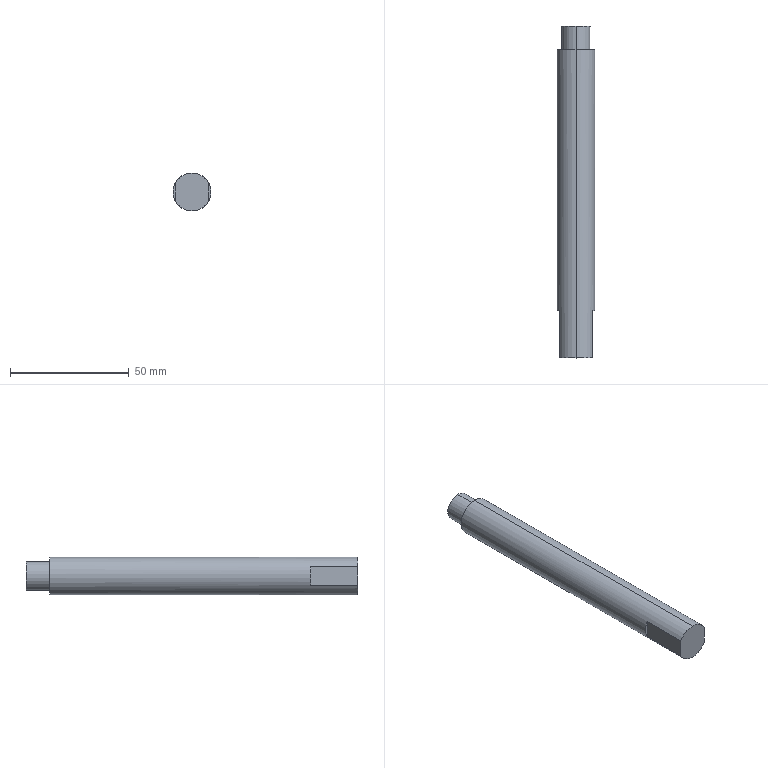Part | SolidWorks | features ICE 2, Extrusion 1, HoleWzd 1 | 1 solid | 11 faces | box 16 x 140 x 16 mm | volume 27060 mm3 | plane 7 | cylinder 4 | commonest cylinder face diameters 12 x2 16 x2
STEP:
#1=CARTESIAN_POINT('',(0.,140.,6.));
#2=VERTEX_POINT('',#1);
#3=CARTESIAN_POINT('',(0.,140.,-6.));
#4=VERTEX_POINT('',#3);
#5=CARTESIAN_POINT('',(0.,140.,0.));
#6=DIRECTION('',(0.,1.,0.));
#7=DIRECTION('',(0.,0.,1.));
#8=AXIS2_PLACEMENT_3D('',#5,#6,#7);
#9=CIRCLE('',#8,6.);
#10=EDGE_CURVE('',#2,#4,#9,.T.);
#11=ORIENTED_EDGE('',*,*,#10,.F.);
#12=CARTESIAN_POINT('',(0.,130.,6.));
#13=VERTEX_POINT('',#12);
#14=CARTESIAN_POINT('',(0.,140.,6.));
#15=DIRECTION('',(0.,-1.,0.));
#16=VECTOR('',#15,1000.);
#17=LINE('',#14,#16);
#18=EDGE_CURVE('',#2,#13,#17,.T.);
#19=ORIENTED_EDGE('',*,*,#18,.T.);
#20=CARTESIAN_POINT('',(0.,130.,-6.));
#21=VERTEX_POINT('',#20);
#22=CARTESIAN_POINT('',(0.,130.,0.));
#23=DIRECTION('',(0.,1.,0.));
#24=DIRECTION('',(0.,0.,1.));
#25=AXIS2_PLACEMENT_3D('',#22,#23,#24);
#26=CIRCLE('',#25,6.);
#27=EDGE_CURVE('',#13,#21,#26,.T.);
#28=ORIENTED_EDGE('',*,*,#27,.T.);
#29=CARTESIAN_POINT('',(0.,140.,-6.));
#30=DIRECTION('',(0.,-1.,0.));
#31=VECTOR('',#30,1000.);
#32=LINE('',#29,#31);
#33=EDGE_CURVE('',#4,#21,#32,.T.);
#34=ORIENTED_EDGE('',*,*,#33,.F.);
#35=EDGE_LOOP('',(#11,#19,#28,#34));
#36=FACE_OUTER_BOUND('',#35,.T.);
#37=CARTESIAN_POINT('',(0.,140.,0.));
#38=DIRECTION('',(0.,-1.,0.));
#39=DIRECTION('',(0.,0.,-1.));
#40=AXIS2_PLACEMENT_3D('',#37,#38,#39);
#41=CYLINDRICAL_SURFACE('',#40,6.);
#42=ADVANCED_FACE('',(#36),#41,.T.);
#43=CARTESIAN_POINT('',(0.,130.,8.));
#44=VERTEX_POINT('',#43);
#45=CARTESIAN_POINT('',(0.,130.,-8.));
#46=VERTEX_POINT('',#45);
#47=CARTESIAN_POINT('',(0.,130.,0.));
#48=DIRECTION('',(0.,1.,0.));
#49=DIRECTION('',(0.,0.,1.));
#50=AXIS2_PLACEMENT_3D('',#47,#48,#49);
#51=CIRCLE('',#50,8.);
#52=EDGE_CURVE('',#44,#46,#51,.T.);
#53=ORIENTED_EDGE('',*,*,#52,.F.);
#54=CARTESIAN_POINT('',(0.,0.,8.));
#55=VERTEX_POINT('',#54);
#56=CARTESIAN_POINT('',(0.,130.,8.));
#57=DIRECTION('',(0.,-1.,0.));
#58=VECTOR('',#57,1000.);
#59=LINE('',#56,#58);
#60=EDGE_CURVE('',#44,#55,#59,.T.);
#61=ORIENTED_EDGE('',*,*,#60,.T.);
#62=CARTESIAN_POINT('',(7.,0.,3.873));
#63=VERTEX_POINT('',#62);
#64=CARTESIAN_POINT('',(0.,0.,0.));
#65=DIRECTION('',(0.,1.,0.));
#66=DIRECTION('',(0.,0.,1.));
#67=AXIS2_PLACEMENT_3D('',#64,#65,#66);
#68=CIRCLE('',#67,8.);
#69=EDGE_CURVE('',#55,#63,#68,.T.);
#70=ORIENTED_EDGE('',*,*,#69,.T.);
#71=CARTESIAN_POINT('',(7.,20.,3.873));
#72=VERTEX_POINT('',#71);
#73=CARTESIAN_POINT('',(7.,130.,3.873));
#74=DIRECTION('',(0.,1.,0.));
#75=VECTOR('',#74,1000.);
#76=LINE('',#73,#75);
#77=EDGE_CURVE('',#63,#72,#76,.T.);
#78=ORIENTED_EDGE('',*,*,#77,.T.);
#79=CARTESIAN_POINT('',(7.,20.,-3.873));
#80=VERTEX_POINT('',#79);
#81=CARTESIAN_POINT('',(0.,20.,0.));
#82=DIRECTION('',(0.,1.,0.));
#83=DIRECTION('',(-1.,0.,0.));
#84=AXIS2_PLACEMENT_3D('',#81,#82,#83);
#85=CIRCLE('',#84,8.);
#86=EDGE_CURVE('',#72,#80,#85,.T.);
#87=ORIENTED_EDGE('',*,*,#86,.T.);
#88=CARTESIAN_POINT('',(7.,0.,-3.873));
#89=VERTEX_POINT('',#88);
#90=CARTESIAN_POINT('',(7.,130.,-3.873));
#91=DIRECTION('',(0.,-1.,0.));
#92=VECTOR('',#91,1000.);
#93=LINE('',#90,#92);
#94=EDGE_CURVE('',#80,#89,#93,.T.);
#95=ORIENTED_EDGE('',*,*,#94,.T.);
#96=CARTESIAN_POINT('',(0.,0.,-8.));
#97=VERTEX_POINT('',#96);
#98=CARTESIAN_POINT('',(0.,0.,0.));
#99=DIRECTION('',(0.,1.,0.));
#100=DIRECTION('',(0.,0.,1.));
#101=AXIS2_PLACEMENT_3D('',#98,#99,#100);
#102=CIRCLE('',#101,8.);
#103=EDGE_CURVE('',#89,#97,#102,.T.);
#104=ORIENTED_EDGE('',*,*,#103,.T.);
#105=CARTESIAN_POINT('',(0.,130.,-8.));
#106=DIRECTION('',(0.,-1.,0.));
#107=VECTOR('',#106,1000.);
#108=LINE('',#105,#107);
#109=EDGE_CURVE('',#46,#97,#108,.T.);
#110=ORIENTED_EDGE('',*,*,#109,.F.);
#111=EDGE_LOOP('',(#53,#61,#70,#78,#87,#95,#104,#110));
#112=FACE_OUTER_BOUND('',#111,.T.);
#113=CARTESIAN_POINT('',(0.,130.,0.));
#114=DIRECTION('',(0.,-1.,0.));
#115=DIRECTION('',(0.,0.,-1.));
#116=AXIS2_PLACEMENT_3D('',#113,#114,#115);
#117=CYLINDRICAL_SURFACE('',#116,8.);
#118=ADVANCED_FACE('',(#112),#117,.T.);
#119=ORIENTED_EDGE('',*,*,#60,.F.);
#120=CARTESIAN_POINT('',(0.,130.,0.));
#121=DIRECTION('',(0.,1.,0.));
#122=DIRECTION('',(0.,0.,1.));
#123=AXIS2_PLACEMENT_3D('',#120,#121,#122);
#124=CIRCLE('',#123,8.);
#125=EDGE_CURVE('',#46,#44,#124,.T.);
#126=ORIENTED_EDGE('',*,*,#125,.F.);
#127=ORIENTED_EDGE('',*,*,#109,.T.);
#128=CARTESIAN_POINT('',(-7.,0.,-3.873));
#129=VERTEX_POINT('',#128);
#130=CARTESIAN_POINT('',(0.,0.,0.));
#131=DIRECTION('',(0.,1.,0.));
#132=DIRECTION('',(0.,0.,1.));
#133=AXIS2_PLACEMENT_3D('',#130,#131,#132);
#134=CIRCLE('',#133,8.);
#135=EDGE_CURVE('',#97,#129,#134,.T.);
#136=ORIENTED_EDGE('',*,*,#135,.T.);
#137=CARTESIAN_POINT('',(-7.,20.,-3.873));
#138=VERTEX_POINT('',#137);
#139=CARTESIAN_POINT('',(-7.,130.,-3.873));
#140=DIRECTION('',(0.,1.,0.));
#141=VECTOR('',#140,1000.);
#142=LINE('',#139,#141);
#143=EDGE_CURVE('',#129,#138,#142,.T.);
#144=ORIENTED_EDGE('',*,*,#143,.T.);
#145=CARTESIAN_POINT('',(-7.,20.,3.873));
#146=VERTEX_POINT('',#145);
#147=CARTESIAN_POINT('',(0.,20.,0.));
#148=DIRECTION('',(0.,1.,0.));
#149=DIRECTION('',(-1.,0.,0.));
#150=AXIS2_PLACEMENT_3D('',#147,#148,#149);
#151=CIRCLE('',#150,8.);
#152=EDGE_CURVE('',#138,#146,#151,.T.);
#153=ORIENTED_EDGE('',*,*,#152,.T.);
#154=CARTESIAN_POINT('',(-7.,0.,3.873));
#155=VERTEX_POINT('',#154);
#156=CARTESIAN_POINT('',(-7.,130.,3.873));
#157=DIRECTION('',(0.,-1.,0.));
#158=VECTOR('',#157,1000.);
#159=LINE('',#156,#158);
#160=EDGE_CURVE('',#146,#155,#159,.T.);
#161=ORIENTED_EDGE('',*,*,#160,.T.);
#162=CARTESIAN_POINT('',(0.,0.,0.));
#163=DIRECTION('',(0.,1.,0.));
#164=DIRECTION('',(0.,0.,1.));
#165=AXIS2_PLACEMENT_3D('',#162,#163,#164);
#166=CIRCLE('',#165,8.);
#167=EDGE_CURVE('',#155,#55,#166,.T.);
#168=ORIENTED_EDGE('',*,*,#167,.T.);
#169=EDGE_LOOP('',(#119,#126,#127,#136,#144,#153,#161,#168));
#170=FACE_OUTER_BOUND('',#169,.T.);
#171=CARTESIAN_POINT('',(0.,130.,0.));
#172=DIRECTION('',(0.,-1.,0.));
#173=DIRECTION('',(0.,0.,-1.));
#174=AXIS2_PLACEMENT_3D('',#171,#172,#173);
#175=CYLINDRICAL_SURFACE('',#174,8.);
#176=ADVANCED_FACE('',(#170),#175,.T.);
#177=CARTESIAN_POINT('',(0.,130.,0.));
#178=DIRECTION('',(0.,1.,0.));
#179=DIRECTION('',(0.,0.,1.));
#180=AXIS2_PLACEMENT_3D('',#177,#178,#179);
#181=CIRCLE('',#180,6.);
#182=EDGE_CURVE('',#21,#13,#181,.T.);
#183=ORIENTED_EDGE('',*,*,#182,.F.);
#184=ORIENTED_EDGE('',*,*,#27,.F.);
#185=EDGE_LOOP('',(#183,#184));
#186=FACE_BOUND('',#185,.T.);
#187=ORIENTED_EDGE('',*,*,#125,.T.);
#188=ORIENTED_EDGE('',*,*,#52,.T.);
#189=EDGE_LOOP('',(#187,#188));
#190=FACE_OUTER_BOUND('',#189,.T.);
#191=CARTESIAN_POINT('',(0.,130.,0.));
#192=DIRECTION('',(0.,1.,0.));
#193=DIRECTION('',(0.,0.,1.));
#194=AXIS2_PLACEMENT_3D('',#191,#192,#193);
#195=PLANE('',#194);
#196=ADVANCED_FACE('',(#186,#190),#195,.T.);
#197=ORIENTED_EDGE('',*,*,#167,.F.);
#198=CARTESIAN_POINT('',(-7.,0.,0.));
#199=DIRECTION('',(0.,0.,-1.));
#200=VECTOR('',#199,1000.);
#201=LINE('',#198,#200);
#202=EDGE_CURVE('',#155,#129,#201,.T.);
#203=ORIENTED_EDGE('',*,*,#202,.T.);
#204=ORIENTED_EDGE('',*,*,#135,.F.);
#205=ORIENTED_EDGE('',*,*,#103,.F.);
#206=CARTESIAN_POINT('',(7.,0.,0.));
#207=DIRECTION('',(0.,0.,1.));
#208=VECTOR('',#207,1000.);
#209=LINE('',#206,#208);
#210=EDGE_CURVE('',#89,#63,#209,.T.);
#211=ORIENTED_EDGE('',*,*,#210,.T.);
#212=ORIENTED_EDGE('',*,*,#69,.F.);
#213=EDGE_LOOP('',(#197,#203,#204,#205,#211,#212));
#214=FACE_OUTER_BOUND('',#213,.T.);
#215=CARTESIAN_POINT('',(0.,0.,0.));
#216=DIRECTION('',(0.,1.,0.));
#217=DIRECTION('',(0.,0.,1.));
#218=AXIS2_PLACEMENT_3D('',#215,#216,#217);
#219=PLANE('',#218);
#220=ADVANCED_FACE('',(#214),#219,.F.);
#221=ORIENTED_EDGE('',*,*,#18,.F.);
#222=CARTESIAN_POINT('',(0.,140.,0.));
#223=DIRECTION('',(0.,1.,0.));
#224=DIRECTION('',(0.,0.,1.));
#225=AXIS2_PLACEMENT_3D('',#222,#223,#224);
#226=CIRCLE('',#225,6.);
#227=EDGE_CURVE('',#4,#2,#226,.T.);
#228=ORIENTED_EDGE('',*,*,#227,.F.);
#229=ORIENTED_EDGE('',*,*,#33,.T.);
#230=ORIENTED_EDGE('',*,*,#182,.T.);
#231=EDGE_LOOP('',(#221,#228,#229,#230));
#232=FACE_OUTER_BOUND('',#231,.T.);
#233=CARTESIAN_POINT('',(0.,140.,0.));
#234=DIRECTION('',(0.,-1.,0.));
#235=DIRECTION('',(0.,0.,-1.));
#236=AXIS2_PLACEMENT_3D('',#233,#234,#235);
#237=CYLINDRICAL_SURFACE('',#236,6.);
#238=ADVANCED_FACE('',(#232),#237,.T.);
#239=ORIENTED_EDGE('',*,*,#227,.T.);
#240=ORIENTED_EDGE('',*,*,#10,.T.);
#241=EDGE_LOOP('',(#239,#240));
#242=FACE_OUTER_BOUND('',#241,.T.);
#243=CARTESIAN_POINT('',(0.,140.,0.));
#244=DIRECTION('',(0.,1.,0.));
#245=DIRECTION('',(0.,0.,1.));
#246=AXIS2_PLACEMENT_3D('',#243,#244,#245);
#247=PLANE('',#246);
#248=ADVANCED_FACE('',(#242),#247,.T.);
#249=CARTESIAN_POINT('',(7.,20.,-5.));
#250=DIRECTION('',(0.,0.,1.));
#251=VECTOR('',#250,1000.);
#252=LINE('',#249,#251);
#253=EDGE_CURVE('',#80,#72,#252,.T.);
#254=ORIENTED_EDGE('',*,*,#253,.F.);
#255=ORIENTED_EDGE('',*,*,#86,.F.);
#256=EDGE_LOOP('',(#254,#255));
#257=FACE_OUTER_BOUND('',#256,.T.);
#258=CARTESIAN_POINT('',(20.423,20.,-5.));
#259=DIRECTION('',(0.,1.,0.));
#260=DIRECTION('',(-1.,0.,0.));
#261=AXIS2_PLACEMENT_3D('',#258,#259,#260);
#262=PLANE('',#261);
#263=ADVANCED_FACE('',(#257),#262,.F.);
#264=ORIENTED_EDGE('',*,*,#253,.T.);
#265=ORIENTED_EDGE('',*,*,#77,.F.);
#266=ORIENTED_EDGE('',*,*,#210,.F.);
#267=ORIENTED_EDGE('',*,*,#94,.F.);
#268=EDGE_LOOP('',(#264,#265,#266,#267));
#269=FACE_OUTER_BOUND('',#268,.T.);
#270=CARTESIAN_POINT('',(7.,-4.946,-5.));
#271=DIRECTION('',(-1.,0.,0.));
#272=DIRECTION('',(0.,-1.,0.));
#273=AXIS2_PLACEMENT_3D('',#270,#271,#272);
#274=PLANE('',#273);
#275=ADVANCED_FACE('',(#269),#274,.F.);
#276=CARTESIAN_POINT('',(-7.,20.,-5.));
#277=DIRECTION('',(0.,0.,1.));
#278=VECTOR('',#277,1000.);
#279=LINE('',#276,#278);
#280=EDGE_CURVE('',#138,#146,#279,.T.);
#281=ORIENTED_EDGE('',*,*,#280,.T.);
#282=ORIENTED_EDGE('',*,*,#152,.F.);
#283=EDGE_LOOP('',(#281,#282));
#284=FACE_OUTER_BOUND('',#283,.T.);
#285=CARTESIAN_POINT('',(-20.237,20.,-5.));
#286=DIRECTION('',(0.,1.,0.));
#287=DIRECTION('',(-1.,0.,0.));
#288=AXIS2_PLACEMENT_3D('',#285,#286,#287);
#289=PLANE('',#288);
#290=ADVANCED_FACE('',(#284),#289,.F.);
#291=ORIENTED_EDGE('',*,*,#280,.F.);
#292=ORIENTED_EDGE('',*,*,#143,.F.);
#293=ORIENTED_EDGE('',*,*,#202,.F.);
#294=ORIENTED_EDGE('',*,*,#160,.F.);
#295=EDGE_LOOP('',(#291,#292,#293,#294));
#296=FACE_OUTER_BOUND('',#295,.T.);
#297=CARTESIAN_POINT('',(-7.,20.,-5.));
#298=DIRECTION('',(1.,0.,0.));
#299=DIRECTION('',(0.,1.,0.));
#300=AXIS2_PLACEMENT_3D('',#297,#298,#299);
#301=PLANE('',#300);
#302=ADVANCED_FACE('',(#296),#301,.F.);
#303=CLOSED_SHELL('',(#42,#118,#176,#196,#220,#238,#248,#263,#275,#290,#302));
#304=MANIFOLD_SOLID_BREP('',#303);
#305=CARTESIAN_POINT('',(0.,0.,0.));
#306=DIRECTION('',(0.,0.,1.));
#307=DIRECTION('',(1.,0.,0.));
#308=AXIS2_PLACEMENT_3D('',#305,#306,#307);
#309=(LENGTH_UNIT()NAMED_UNIT(*)SI_UNIT(.MILLI.,.METRE.));
#310=UNCERTAINTY_MEASURE_WITH_UNIT(LENGTH_MEASURE(0.00001),#309,'','');
#311=(NAMED_UNIT(*)PLANE_ANGLE_UNIT()SI_UNIT($,.RADIAN.));
#312=(NAMED_UNIT(*)SI_UNIT($,.STERADIAN.)SOLID_ANGLE_UNIT());
#313=(GEOMETRIC_REPRESENTATION_CONTEXT(3)GLOBAL_UNCERTAINTY_ASSIGNED_CONTEXT((#310))GLOBAL_UNIT_ASSIGNED_CONTEXT((#309,#311,#312))REPRESENTATION_CONTEXT('',''));
#314=ADVANCED_BREP_SHAPE_REPRESENTATION('',(#304,#308),#313);